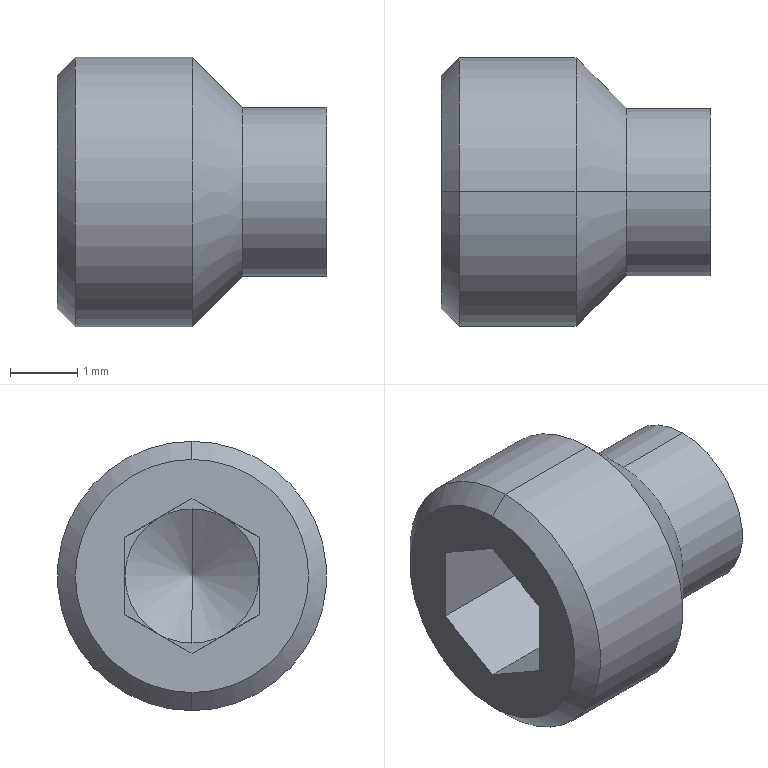Part | STEP file | 1 solid | 24 faces | box 4 x 4 x 4 mm | volume 31.419 mm3 | plane 14 | cone 6 | cylinder 4 | commonest cylinder face diameters 2.5 x2 4 x2